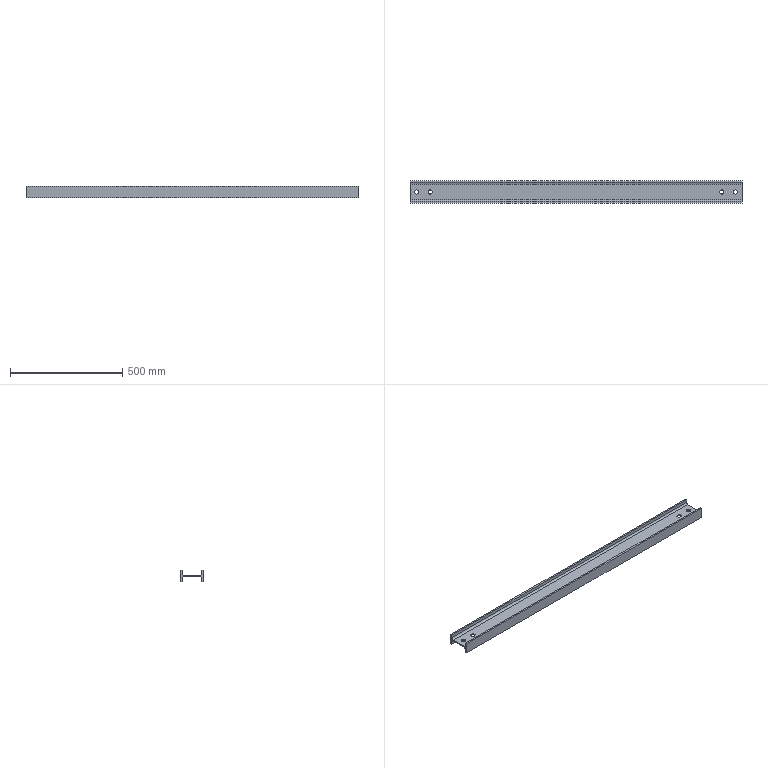Part | STEP file | Electrical cabinet walkway secondary beam 1 body_Default<As Machined> | 1 solid | 26 faces | box 1480 x 100 x 50 mm | volume 1748038 mm3 | plane 14 | cylinder 12 | commonest cylinder face diameters 19 x8 16 x4